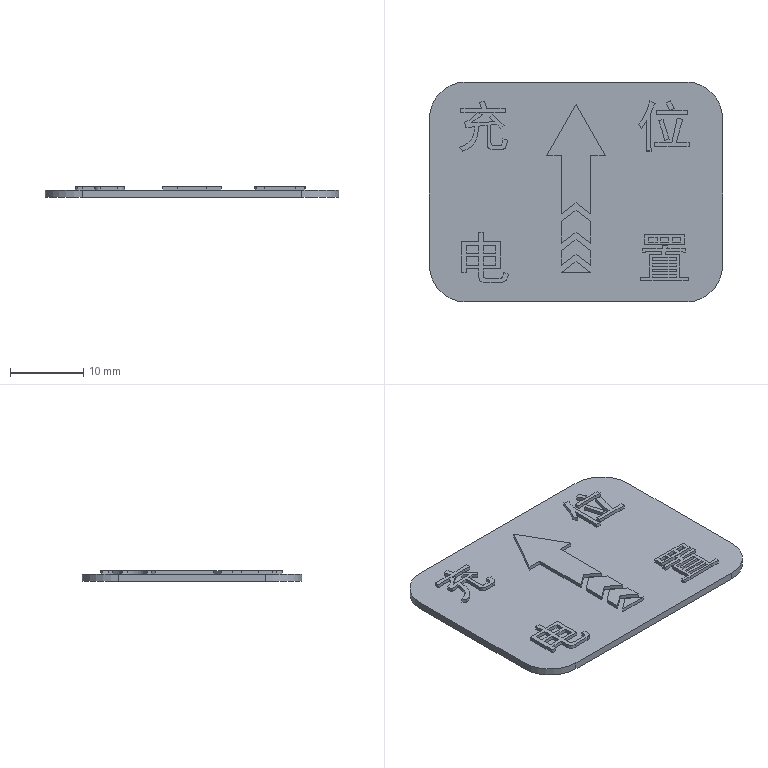Part | SolidWorks | features BaseBody 1 | 1 solid | 233 faces | box 40 x 30 x 1.5 mm | volume 1250 mm3 | plane 149 | spline 80 | cylinder 4 | commonest cylinder face diameters 10 x4